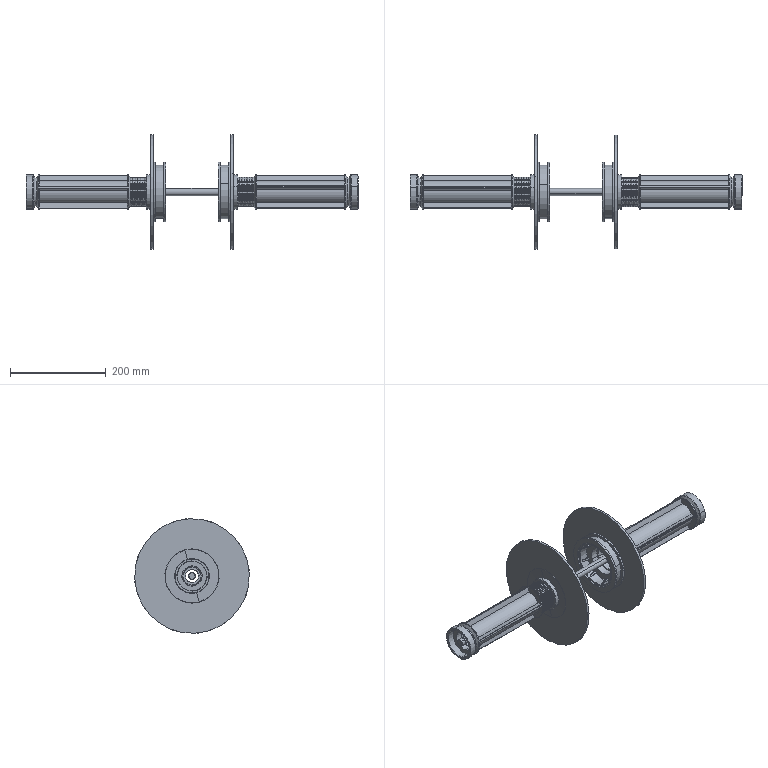Part | SolidWorks | features CompositeCurve 3 | 7 solids | 574 faces | box 694.8 x 240 x 240 mm | volume 1341912 mm3 | cylinder 232 | torus 144 | plane 106 | cone 84 | spline 8 | commonest cylinder face diameters 60.4 x92 1 x56 15 x10 14.3 x8 42.38 x8 48 x8